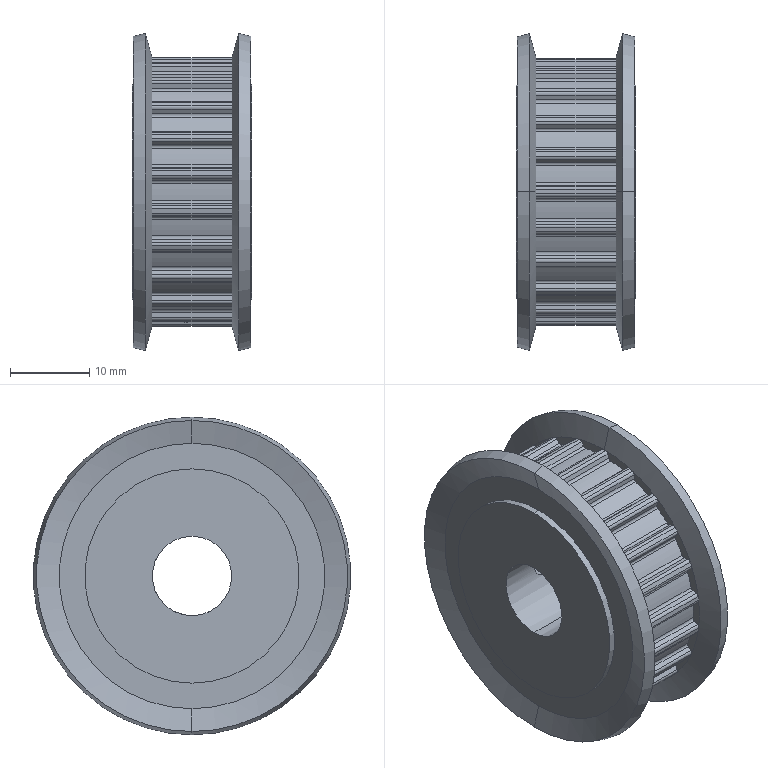Part | STEP file | Synchronous wheel TTPA22-AT5100-A-P10_b V1.201001 | 1 solid | 253 faces | box 15 x 40 x 40 mm | volume 11899 mm3 | cylinder 149 | plane 92 | cone 12 | commonest cylinder face diameters 0.8 x92 31.65 x24 33.85 x23 3.242 x4 27 x4 10 x2